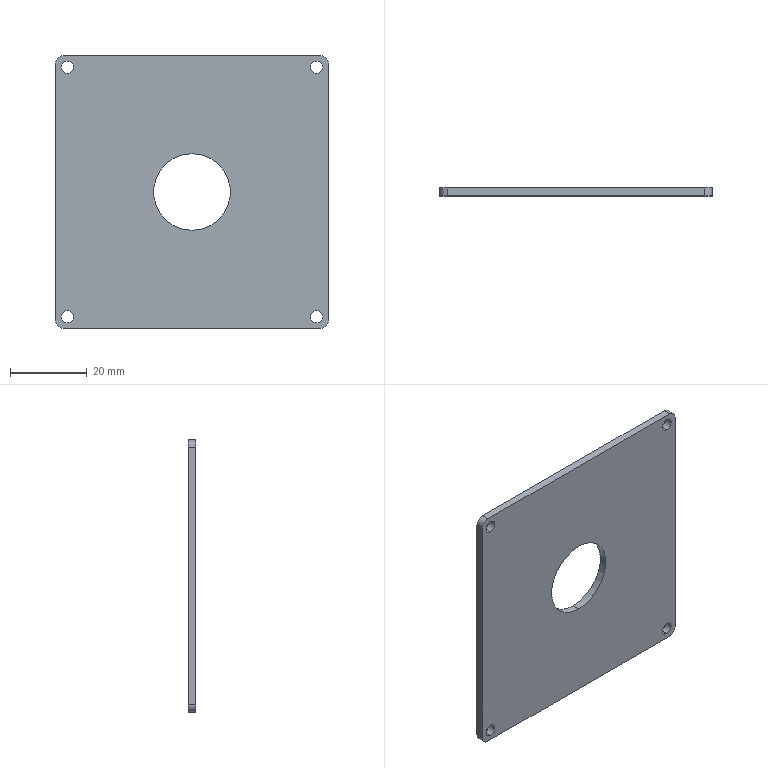Part | SolidWorks | features Extrusion 1, ICE 1 | 1 solid | 20 faces | box 71 x 2 x 71 mm | volume 9382 mm3 | cylinder 14 | plane 6 | commonest cylinder face diameters 3.2 x8 4 x4 20 x2
STEP:
#1=CARTESIAN_POINT('',(0.,0.,10.));
#2=VERTEX_POINT('',#1);
#3=CARTESIAN_POINT('',(0.,0.,-10.));
#4=VERTEX_POINT('',#3);
#5=CARTESIAN_POINT('',(0.,0.,0.));
#6=DIRECTION('',(0.,-1.,0.));
#7=DIRECTION('',(0.,0.,-1.));
#8=AXIS2_PLACEMENT_3D('',#5,#6,#7);
#9=CIRCLE('',#8,10.);
#10=EDGE_CURVE('',#2,#4,#9,.T.);
#11=ORIENTED_EDGE('',*,*,#10,.T.);
#12=CARTESIAN_POINT('',(0.,2.,-10.));
#13=VERTEX_POINT('',#12);
#14=CARTESIAN_POINT('',(0.,-8.,-10.));
#15=DIRECTION('',(0.,1.,0.));
#16=VECTOR('',#15,1000.);
#17=LINE('',#14,#16);
#18=EDGE_CURVE('',#4,#13,#17,.T.);
#19=ORIENTED_EDGE('',*,*,#18,.T.);
#20=CARTESIAN_POINT('',(0.,2.,10.));
#21=VERTEX_POINT('',#20);
#22=CARTESIAN_POINT('',(0.,2.,0.));
#23=DIRECTION('',(0.,1.,0.));
#24=DIRECTION('',(0.,0.,1.));
#25=AXIS2_PLACEMENT_3D('',#22,#23,#24);
#26=CIRCLE('',#25,10.);
#27=EDGE_CURVE('',#13,#21,#26,.T.);
#28=ORIENTED_EDGE('',*,*,#27,.T.);
#29=CARTESIAN_POINT('',(0.,-8.,10.));
#30=DIRECTION('',(0.,1.,0.));
#31=VECTOR('',#30,1000.);
#32=LINE('',#29,#31);
#33=EDGE_CURVE('',#2,#21,#32,.T.);
#34=ORIENTED_EDGE('',*,*,#33,.F.);
#35=EDGE_LOOP('',(#11,#19,#28,#34));
#36=FACE_OUTER_BOUND('',#35,.T.);
#37=CARTESIAN_POINT('',(0.,-8.,0.));
#38=DIRECTION('',(0.,1.,0.));
#39=DIRECTION('',(0.,0.,1.));
#40=AXIS2_PLACEMENT_3D('',#37,#38,#39);
#41=CYLINDRICAL_SURFACE('',#40,10.);
#42=ADVANCED_FACE('',(#36),#41,.F.);
#43=CARTESIAN_POINT('',(-32.5,2.,30.9));
#44=VERTEX_POINT('',#43);
#45=CARTESIAN_POINT('',(-32.5,2.,34.1));
#46=VERTEX_POINT('',#45);
#47=CARTESIAN_POINT('',(-32.5,2.,32.5));
#48=DIRECTION('',(0.,1.,0.));
#49=DIRECTION('',(0.,0.,1.));
#50=AXIS2_PLACEMENT_3D('',#47,#48,#49);
#51=CIRCLE('',#50,1.6);
#52=EDGE_CURVE('',#44,#46,#51,.T.);
#53=ORIENTED_EDGE('',*,*,#52,.T.);
#54=CARTESIAN_POINT('',(-32.5,0.,34.1));
#55=VERTEX_POINT('',#54);
#56=CARTESIAN_POINT('',(-32.5,2.,34.1));
#57=DIRECTION('',(0.,-1.,0.));
#58=VECTOR('',#57,1000.);
#59=LINE('',#56,#58);
#60=EDGE_CURVE('',#46,#55,#59,.T.);
#61=ORIENTED_EDGE('',*,*,#60,.T.);
#62=CARTESIAN_POINT('',(-32.5,0.,30.9));
#63=VERTEX_POINT('',#62);
#64=CARTESIAN_POINT('',(-32.5,0.,32.5));
#65=DIRECTION('',(0.,1.,0.));
#66=DIRECTION('',(0.,0.,1.));
#67=AXIS2_PLACEMENT_3D('',#64,#65,#66);
#68=CIRCLE('',#67,1.6);
#69=EDGE_CURVE('',#63,#55,#68,.T.);
#70=ORIENTED_EDGE('',*,*,#69,.F.);
#71=CARTESIAN_POINT('',(-32.5,2.,30.9));
#72=DIRECTION('',(0.,-1.,0.));
#73=VECTOR('',#72,1000.);
#74=LINE('',#71,#73);
#75=EDGE_CURVE('',#44,#63,#74,.T.);
#76=ORIENTED_EDGE('',*,*,#75,.F.);
#77=EDGE_LOOP('',(#53,#61,#70,#76));
#78=FACE_OUTER_BOUND('',#77,.T.);
#79=CARTESIAN_POINT('',(-32.5,2.,32.5));
#80=DIRECTION('',(0.,-1.,0.));
#81=DIRECTION('',(0.,0.,-1.));
#82=AXIS2_PLACEMENT_3D('',#79,#80,#81);
#83=CYLINDRICAL_SURFACE('',#82,1.6);
#84=ADVANCED_FACE('',(#78),#83,.F.);
#85=CARTESIAN_POINT('',(32.5,2.,30.9));
#86=VERTEX_POINT('',#85);
#87=CARTESIAN_POINT('',(32.5,2.,34.1));
#88=VERTEX_POINT('',#87);
#89=CARTESIAN_POINT('',(32.5,2.,32.5));
#90=DIRECTION('',(0.,1.,0.));
#91=DIRECTION('',(0.,0.,1.));
#92=AXIS2_PLACEMENT_3D('',#89,#90,#91);
#93=CIRCLE('',#92,1.6);
#94=EDGE_CURVE('',#86,#88,#93,.T.);
#95=ORIENTED_EDGE('',*,*,#94,.T.);
#96=CARTESIAN_POINT('',(32.5,0.,34.1));
#97=VERTEX_POINT('',#96);
#98=CARTESIAN_POINT('',(32.5,2.,34.1));
#99=DIRECTION('',(0.,-1.,0.));
#100=VECTOR('',#99,1000.);
#101=LINE('',#98,#100);
#102=EDGE_CURVE('',#88,#97,#101,.T.);
#103=ORIENTED_EDGE('',*,*,#102,.T.);
#104=CARTESIAN_POINT('',(32.5,0.,30.9));
#105=VERTEX_POINT('',#104);
#106=CARTESIAN_POINT('',(32.5,0.,32.5));
#107=DIRECTION('',(0.,1.,0.));
#108=DIRECTION('',(0.,0.,1.));
#109=AXIS2_PLACEMENT_3D('',#106,#107,#108);
#110=CIRCLE('',#109,1.6);
#111=EDGE_CURVE('',#105,#97,#110,.T.);
#112=ORIENTED_EDGE('',*,*,#111,.F.);
#113=CARTESIAN_POINT('',(32.5,2.,30.9));
#114=DIRECTION('',(0.,-1.,0.));
#115=VECTOR('',#114,1000.);
#116=LINE('',#113,#115);
#117=EDGE_CURVE('',#86,#105,#116,.T.);
#118=ORIENTED_EDGE('',*,*,#117,.F.);
#119=EDGE_LOOP('',(#95,#103,#112,#118));
#120=FACE_OUTER_BOUND('',#119,.T.);
#121=CARTESIAN_POINT('',(32.5,2.,32.5));
#122=DIRECTION('',(0.,-1.,0.));
#123=DIRECTION('',(0.,0.,-1.));
#124=AXIS2_PLACEMENT_3D('',#121,#122,#123);
#125=CYLINDRICAL_SURFACE('',#124,1.6);
#126=ADVANCED_FACE('',(#120),#125,.F.);
#127=CARTESIAN_POINT('',(32.5,2.,-34.1));
#128=VERTEX_POINT('',#127);
#129=CARTESIAN_POINT('',(32.5,2.,-30.9));
#130=VERTEX_POINT('',#129);
#131=CARTESIAN_POINT('',(32.5,2.,-32.5));
#132=DIRECTION('',(0.,1.,0.));
#133=DIRECTION('',(0.,0.,1.));
#134=AXIS2_PLACEMENT_3D('',#131,#132,#133);
#135=CIRCLE('',#134,1.6);
#136=EDGE_CURVE('',#128,#130,#135,.T.);
#137=ORIENTED_EDGE('',*,*,#136,.T.);
#138=CARTESIAN_POINT('',(32.5,0.,-30.9));
#139=VERTEX_POINT('',#138);
#140=CARTESIAN_POINT('',(32.5,2.,-30.9));
#141=DIRECTION('',(0.,-1.,0.));
#142=VECTOR('',#141,1000.);
#143=LINE('',#140,#142);
#144=EDGE_CURVE('',#130,#139,#143,.T.);
#145=ORIENTED_EDGE('',*,*,#144,.T.);
#146=CARTESIAN_POINT('',(32.5,0.,-34.1));
#147=VERTEX_POINT('',#146);
#148=CARTESIAN_POINT('',(32.5,0.,-32.5));
#149=DIRECTION('',(0.,1.,0.));
#150=DIRECTION('',(0.,0.,1.));
#151=AXIS2_PLACEMENT_3D('',#148,#149,#150);
#152=CIRCLE('',#151,1.6);
#153=EDGE_CURVE('',#147,#139,#152,.T.);
#154=ORIENTED_EDGE('',*,*,#153,.F.);
#155=CARTESIAN_POINT('',(32.5,2.,-34.1));
#156=DIRECTION('',(0.,-1.,0.));
#157=VECTOR('',#156,1000.);
#158=LINE('',#155,#157);
#159=EDGE_CURVE('',#128,#147,#158,.T.);
#160=ORIENTED_EDGE('',*,*,#159,.F.);
#161=EDGE_LOOP('',(#137,#145,#154,#160));
#162=FACE_OUTER_BOUND('',#161,.T.);
#163=CARTESIAN_POINT('',(32.5,2.,-32.5));
#164=DIRECTION('',(0.,-1.,0.));
#165=DIRECTION('',(0.,0.,-1.));
#166=AXIS2_PLACEMENT_3D('',#163,#164,#165);
#167=CYLINDRICAL_SURFACE('',#166,1.6);
#168=ADVANCED_FACE('',(#162),#167,.F.);
#169=CARTESIAN_POINT('',(-32.5,2.,-34.1));
#170=VERTEX_POINT('',#169);
#171=CARTESIAN_POINT('',(-32.5,2.,-30.9));
#172=VERTEX_POINT('',#171);
#173=CARTESIAN_POINT('',(-32.5,2.,-32.5));
#174=DIRECTION('',(0.,1.,0.));
#175=DIRECTION('',(0.,0.,1.));
#176=AXIS2_PLACEMENT_3D('',#173,#174,#175);
#177=CIRCLE('',#176,1.6);
#178=EDGE_CURVE('',#170,#172,#177,.T.);
#179=ORIENTED_EDGE('',*,*,#178,.T.);
#180=CARTESIAN_POINT('',(-32.5,0.,-30.9));
#181=VERTEX_POINT('',#180);
#182=CARTESIAN_POINT('',(-32.5,2.,-30.9));
#183=DIRECTION('',(0.,-1.,0.));
#184=VECTOR('',#183,1000.);
#185=LINE('',#182,#184);
#186=EDGE_CURVE('',#172,#181,#185,.T.);
#187=ORIENTED_EDGE('',*,*,#186,.T.);
#188=CARTESIAN_POINT('',(-32.5,0.,-34.1));
#189=VERTEX_POINT('',#188);
#190=CARTESIAN_POINT('',(-32.5,0.,-32.5));
#191=DIRECTION('',(0.,1.,0.));
#192=DIRECTION('',(0.,0.,1.));
#193=AXIS2_PLACEMENT_3D('',#190,#191,#192);
#194=CIRCLE('',#193,1.6);
#195=EDGE_CURVE('',#189,#181,#194,.T.);
#196=ORIENTED_EDGE('',*,*,#195,.F.);
#197=CARTESIAN_POINT('',(-32.5,2.,-34.1));
#198=DIRECTION('',(0.,-1.,0.));
#199=VECTOR('',#198,1000.);
#200=LINE('',#197,#199);
#201=EDGE_CURVE('',#170,#189,#200,.T.);
#202=ORIENTED_EDGE('',*,*,#201,.F.);
#203=EDGE_LOOP('',(#179,#187,#196,#202));
#204=FACE_OUTER_BOUND('',#203,.T.);
#205=CARTESIAN_POINT('',(-32.5,2.,-32.5));
#206=DIRECTION('',(0.,-1.,0.));
#207=DIRECTION('',(0.,0.,-1.));
#208=AXIS2_PLACEMENT_3D('',#205,#206,#207);
#209=CYLINDRICAL_SURFACE('',#208,1.6);
#210=ADVANCED_FACE('',(#204),#209,.F.);
#211=CARTESIAN_POINT('',(0.,2.,0.));
#212=DIRECTION('',(0.,1.,0.));
#213=DIRECTION('',(0.,0.,1.));
#214=AXIS2_PLACEMENT_3D('',#211,#212,#213);
#215=CIRCLE('',#214,10.);
#216=EDGE_CURVE('',#21,#13,#215,.T.);
#217=ORIENTED_EDGE('',*,*,#216,.F.);
#218=ORIENTED_EDGE('',*,*,#27,.F.);
#219=EDGE_LOOP('',(#217,#218));
#220=FACE_BOUND('',#219,.T.);
#221=CARTESIAN_POINT('',(-35.5,2.,33.5));
#222=VERTEX_POINT('',#221);
#223=CARTESIAN_POINT('',(-33.5,2.,35.5));
#224=VERTEX_POINT('',#223);
#225=CARTESIAN_POINT('',(-33.5,2.,33.5));
#226=DIRECTION('',(0.,1.,0.));
#227=DIRECTION('',(0.,0.,-1.));
#228=AXIS2_PLACEMENT_3D('',#225,#226,#227);
#229=CIRCLE('',#228,2.);
#230=EDGE_CURVE('',#222,#224,#229,.T.);
#231=ORIENTED_EDGE('',*,*,#230,.T.);
#232=CARTESIAN_POINT('',(33.5,2.,35.5));
#233=VERTEX_POINT('',#232);
#234=CARTESIAN_POINT('',(-33.5,2.,35.5));
#235=DIRECTION('',(1.,0.,0.));
#236=VECTOR('',#235,1000.);
#237=LINE('',#234,#236);
#238=EDGE_CURVE('',#224,#233,#237,.T.);
#239=ORIENTED_EDGE('',*,*,#238,.T.);
#240=CARTESIAN_POINT('',(35.5,2.,33.5));
#241=VERTEX_POINT('',#240);
#242=CARTESIAN_POINT('',(33.5,2.,33.5));
#243=DIRECTION('',(0.,1.,0.));
#244=DIRECTION('',(0.,0.,1.));
#245=AXIS2_PLACEMENT_3D('',#242,#243,#244);
#246=CIRCLE('',#245,2.);
#247=EDGE_CURVE('',#233,#241,#246,.T.);
#248=ORIENTED_EDGE('',*,*,#247,.T.);
#249=CARTESIAN_POINT('',(35.5,2.,-33.5));
#250=VERTEX_POINT('',#249);
#251=CARTESIAN_POINT('',(35.5,2.,33.5));
#252=DIRECTION('',(0.,0.,-1.));
#253=VECTOR('',#252,1000.);
#254=LINE('',#251,#253);
#255=EDGE_CURVE('',#241,#250,#254,.T.);
#256=ORIENTED_EDGE('',*,*,#255,.T.);
#257=CARTESIAN_POINT('',(33.5,2.,-35.5));
#258=VERTEX_POINT('',#257);
#259=CARTESIAN_POINT('',(33.5,2.,-33.5));
#260=DIRECTION('',(0.,1.,0.));
#261=DIRECTION('',(0.,0.,-1.));
#262=AXIS2_PLACEMENT_3D('',#259,#260,#261);
#263=CIRCLE('',#262,2.);
#264=EDGE_CURVE('',#250,#258,#263,.T.);
#265=ORIENTED_EDGE('',*,*,#264,.T.);
#266=CARTESIAN_POINT('',(-33.5,2.,-35.5));
#267=VERTEX_POINT('',#266);
#268=CARTESIAN_POINT('',(-33.5,2.,-35.5));
#269=DIRECTION('',(-1.,0.,0.));
#270=VECTOR('',#269,1000.);
#271=LINE('',#268,#270);
#272=EDGE_CURVE('',#258,#267,#271,.T.);
#273=ORIENTED_EDGE('',*,*,#272,.T.);
#274=CARTESIAN_POINT('',(-35.5,2.,-33.5));
#275=VERTEX_POINT('',#274);
#276=CARTESIAN_POINT('',(-33.5,2.,-33.5));
#277=DIRECTION('',(0.,1.,0.));
#278=DIRECTION('',(0.,0.,-1.));
#279=AXIS2_PLACEMENT_3D('',#276,#277,#278);
#280=CIRCLE('',#279,2.);
#281=EDGE_CURVE('',#267,#275,#280,.T.);
#282=ORIENTED_EDGE('',*,*,#281,.T.);
#283=CARTESIAN_POINT('',(-35.5,2.,33.5));
#284=DIRECTION('',(0.,0.,1.));
#285=VECTOR('',#284,1000.);
#286=LINE('',#283,#285);
#287=EDGE_CURVE('',#275,#222,#286,.T.);
#288=ORIENTED_EDGE('',*,*,#287,.T.);
#289=EDGE_LOOP('',(#231,#239,#248,#256,#265,#273,#282,#288));
#290=FACE_OUTER_BOUND('',#289,.T.);
#291=ORIENTED_EDGE('',*,*,#178,.F.);
#292=CARTESIAN_POINT('',(-32.5,2.,-32.5));
#293=DIRECTION('',(0.,1.,0.));
#294=DIRECTION('',(0.,0.,1.));
#295=AXIS2_PLACEMENT_3D('',#292,#293,#294);
#296=CIRCLE('',#295,1.6);
#297=EDGE_CURVE('',#172,#170,#296,.T.);
#298=ORIENTED_EDGE('',*,*,#297,.F.);
#299=EDGE_LOOP('',(#291,#298));
#300=FACE_BOUND('',#299,.T.);
#301=ORIENTED_EDGE('',*,*,#136,.F.);
#302=CARTESIAN_POINT('',(32.5,2.,-32.5));
#303=DIRECTION('',(0.,1.,0.));
#304=DIRECTION('',(0.,0.,1.));
#305=AXIS2_PLACEMENT_3D('',#302,#303,#304);
#306=CIRCLE('',#305,1.6);
#307=EDGE_CURVE('',#130,#128,#306,.T.);
#308=ORIENTED_EDGE('',*,*,#307,.F.);
#309=EDGE_LOOP('',(#301,#308));
#310=FACE_BOUND('',#309,.T.);
#311=ORIENTED_EDGE('',*,*,#94,.F.);
#312=CARTESIAN_POINT('',(32.5,2.,32.5));
#313=DIRECTION('',(0.,1.,0.));
#314=DIRECTION('',(0.,0.,1.));
#315=AXIS2_PLACEMENT_3D('',#312,#313,#314);
#316=CIRCLE('',#315,1.6);
#317=EDGE_CURVE('',#88,#86,#316,.T.);
#318=ORIENTED_EDGE('',*,*,#317,.F.);
#319=EDGE_LOOP('',(#311,#318));
#320=FACE_BOUND('',#319,.T.);
#321=ORIENTED_EDGE('',*,*,#52,.F.);
#322=CARTESIAN_POINT('',(-32.5,2.,32.5));
#323=DIRECTION('',(0.,1.,0.));
#324=DIRECTION('',(0.,0.,1.));
#325=AXIS2_PLACEMENT_3D('',#322,#323,#324);
#326=CIRCLE('',#325,1.6);
#327=EDGE_CURVE('',#46,#44,#326,.T.);
#328=ORIENTED_EDGE('',*,*,#327,.F.);
#329=EDGE_LOOP('',(#321,#328));
#330=FACE_BOUND('',#329,.T.);
#331=CARTESIAN_POINT('',(-33.5,2.,33.5));
#332=DIRECTION('',(0.,-1.,0.));
#333=DIRECTION('',(0.,0.,-1.));
#334=AXIS2_PLACEMENT_3D('',#331,#332,#333);
#335=PLANE('',#334);
#336=ADVANCED_FACE('',(#220,#290,#300,#310,#320,#330),#335,.F.);
#337=ORIENTED_EDGE('',*,*,#10,.F.);
#338=CARTESIAN_POINT('',(0.,0.,0.));
#339=DIRECTION('',(0.,-1.,0.));
#340=DIRECTION('',(0.,0.,-1.));
#341=AXIS2_PLACEMENT_3D('',#338,#339,#340);
#342=CIRCLE('',#341,10.);
#343=EDGE_CURVE('',#4,#2,#342,.T.);
#344=ORIENTED_EDGE('',*,*,#343,.F.);
#345=EDGE_LOOP('',(#337,#344));
#346=FACE_BOUND('',#345,.T.);
#347=ORIENTED_EDGE('',*,*,#111,.T.);
#348=CARTESIAN_POINT('',(32.5,0.,32.5));
#349=DIRECTION('',(0.,1.,0.));
#350=DIRECTION('',(0.,0.,1.));
#351=AXIS2_PLACEMENT_3D('',#348,#349,#350);
#352=CIRCLE('',#351,1.6);
#353=EDGE_CURVE('',#97,#105,#352,.T.);
#354=ORIENTED_EDGE('',*,*,#353,.T.);
#355=EDGE_LOOP('',(#347,#354));
#356=FACE_BOUND('',#355,.T.);
#357=ORIENTED_EDGE('',*,*,#195,.T.);
#358=CARTESIAN_POINT('',(-32.5,0.,-32.5));
#359=DIRECTION('',(0.,1.,0.));
#360=DIRECTION('',(0.,0.,1.));
#361=AXIS2_PLACEMENT_3D('',#358,#359,#360);
#362=CIRCLE('',#361,1.6);
#363=EDGE_CURVE('',#181,#189,#362,.T.);
#364=ORIENTED_EDGE('',*,*,#363,.T.);
#365=EDGE_LOOP('',(#357,#364));
#366=FACE_BOUND('',#365,.T.);
#367=CARTESIAN_POINT('',(-35.5,0.,33.5));
#368=VERTEX_POINT('',#367);
#369=CARTESIAN_POINT('',(-33.5,0.,35.5));
#370=VERTEX_POINT('',#369);
#371=CARTESIAN_POINT('',(-33.5,0.,33.5));
#372=DIRECTION('',(0.,1.,0.));
#373=DIRECTION('',(0.,0.,-1.));
#374=AXIS2_PLACEMENT_3D('',#371,#372,#373);
#375=CIRCLE('',#374,2.);
#376=EDGE_CURVE('',#368,#370,#375,.T.);
#377=ORIENTED_EDGE('',*,*,#376,.F.);
#378=CARTESIAN_POINT('',(-35.5,0.,-33.5));
#379=VERTEX_POINT('',#378);
#380=CARTESIAN_POINT('',(-35.5,0.,33.5));
#381=DIRECTION('',(0.,0.,1.));
#382=VECTOR('',#381,1000.);
#383=LINE('',#380,#382);
#384=EDGE_CURVE('',#379,#368,#383,.T.);
#385=ORIENTED_EDGE('',*,*,#384,.F.);
#386=CARTESIAN_POINT('',(-33.5,0.,-35.5));
#387=VERTEX_POINT('',#386);
#388=CARTESIAN_POINT('',(-33.5,0.,-33.5));
#389=DIRECTION('',(0.,1.,0.));
#390=DIRECTION('',(0.,0.,-1.));
#391=AXIS2_PLACEMENT_3D('',#388,#389,#390);
#392=CIRCLE('',#391,2.);
#393=EDGE_CURVE('',#387,#379,#392,.T.);
#394=ORIENTED_EDGE('',*,*,#393,.F.);
#395=CARTESIAN_POINT('',(33.5,0.,-35.5));
#396=VERTEX_POINT('',#395);
#397=CARTESIAN_POINT('',(-33.5,0.,-35.5));
#398=DIRECTION('',(-1.,0.,0.));
#399=VECTOR('',#398,1000.);
#400=LINE('',#397,#399);
#401=EDGE_CURVE('',#396,#387,#400,.T.);
#402=ORIENTED_EDGE('',*,*,#401,.F.);
#403=CARTESIAN_POINT('',(35.5,0.,-33.5));
#404=VERTEX_POINT('',#403);
#405=CARTESIAN_POINT('',(33.5,0.,-33.5));
#406=DIRECTION('',(0.,1.,0.));
#407=DIRECTION('',(0.,0.,-1.));
#408=AXIS2_PLACEMENT_3D('',#405,#406,#407);
#409=CIRCLE('',#408,2.);
#410=EDGE_CURVE('',#404,#396,#409,.T.);
#411=ORIENTED_EDGE('',*,*,#410,.F.);
#412=CARTESIAN_POINT('',(35.5,0.,33.5));
#413=VERTEX_POINT('',#412);
#414=CARTESIAN_POINT('',(35.5,0.,33.5));
#415=DIRECTION('',(0.,0.,-1.));
#416=VECTOR('',#415,1000.);
#417=LINE('',#414,#416);
#418=EDGE_CURVE('',#413,#404,#417,.T.);
#419=ORIENTED_EDGE('',*,*,#418,.F.);
#420=CARTESIAN_POINT('',(33.5,0.,35.5));
#421=VERTEX_POINT('',#420);
#422=CARTESIAN_POINT('',(33.5,0.,33.5));
#423=DIRECTION('',(0.,1.,0.));
#424=DIRECTION('',(0.,0.,1.));
#425=AXIS2_PLACEMENT_3D('',#422,#423,#424);
#426=CIRCLE('',#425,2.);
#427=EDGE_CURVE('',#421,#413,#426,.T.);
#428=ORIENTED_EDGE('',*,*,#427,.F.);
#429=CARTESIAN_POINT('',(-33.5,0.,35.5));
#430=DIRECTION('',(1.,0.,0.));
#431=VECTOR('',#430,1000.);
#432=LINE('',#429,#431);
#433=EDGE_CURVE('',#370,#421,#432,.T.);
#434=ORIENTED_EDGE('',*,*,#433,.F.);
#435=EDGE_LOOP('',(#377,#385,#394,#402,#411,#419,#428,#434));
#436=FACE_OUTER_BOUND('',#435,.T.);
#437=ORIENTED_EDGE('',*,*,#153,.T.);
#438=CARTESIAN_POINT('',(32.5,0.,-32.5));
#439=DIRECTION('',(0.,1.,0.));
#440=DIRECTION('',(0.,0.,1.));
#441=AXIS2_PLACEMENT_3D('',#438,#439,#440);
#442=CIRCLE('',#441,1.6);
#443=EDGE_CURVE('',#139,#147,#442,.T.);
#444=ORIENTED_EDGE('',*,*,#443,.T.);
#445=EDGE_LOOP('',(#437,#444));
#446=FACE_BOUND('',#445,.T.);
#447=ORIENTED_EDGE('',*,*,#69,.T.);
#448=CARTESIAN_POINT('',(-32.5,0.,32.5));
#449=DIRECTION('',(0.,1.,0.));
#450=DIRECTION('',(0.,0.,1.));
#451=AXIS2_PLACEMENT_3D('',#448,#449,#450);
#452=CIRCLE('',#451,1.6);
#453=EDGE_CURVE('',#55,#63,#452,.T.);
#454=ORIENTED_EDGE('',*,*,#453,.T.);
#455=EDGE_LOOP('',(#447,#454));
#456=FACE_BOUND('',#455,.T.);
#457=CARTESIAN_POINT('',(-33.5,0.,33.5));
#458=DIRECTION('',(0.,-1.,0.));
#459=DIRECTION('',(0.,0.,-1.));
#460=AXIS2_PLACEMENT_3D('',#457,#458,#459);
#461=PLANE('',#460);
#462=ADVANCED_FACE('',(#346,#356,#366,#436,#446,#456),#461,.T.);
#463=ORIENTED_EDGE('',*,*,#376,.T.);
#464=CARTESIAN_POINT('',(-33.5,2.,35.5));
#465=DIRECTION('',(0.,-1.,0.));
#466=VECTOR('',#465,1000.);
#467=LINE('',#464,#466);
#468=EDGE_CURVE('',#224,#370,#467,.T.);
#469=ORIENTED_EDGE('',*,*,#468,.F.);
#470=ORIENTED_EDGE('',*,*,#230,.F.);
#471=CARTESIAN_POINT('',(-35.5,2.,33.5));
#472=DIRECTION('',(0.,-1.,0.));
#473=VECTOR('',#472,1000.);
#474=LINE('',#471,#473);
#475=EDGE_CURVE('',#222,#368,#474,.T.);
#476=ORIENTED_EDGE('',*,*,#475,.T.);
#477=EDGE_LOOP('',(#463,#469,#470,#476));
#478=FACE_OUTER_BOUND('',#477,.T.);
#479=CARTESIAN_POINT('',(-33.5,2.,33.5));
#480=DIRECTION('',(0.,-1.,0.));
#481=DIRECTION('',(0.,0.,-1.));
#482=AXIS2_PLACEMENT_3D('',#479,#480,#481);
#483=CYLINDRICAL_SURFACE('',#482,2.);
#484=ADVANCED_FACE('',(#478),#483,.T.);
#485=ORIENTED_EDGE('',*,*,#433,.T.);
#486=CARTESIAN_POINT('',(33.5,2.,35.5));
#487=DIRECTION('',(0.,-1.,0.));
#488=VECTOR('',#487,1000.);
#489=LINE('',#486,#488);
#490=EDGE_CURVE('',#233,#421,#489,.T.);
#491=ORIENTED_EDGE('',*,*,#490,.F.);
#492=ORIENTED_EDGE('',*,*,#238,.F.);
#493=ORIENTED_EDGE('',*,*,#468,.T.);
#494=EDGE_LOOP('',(#485,#491,#492,#493));
#495=FACE_OUTER_BOUND('',#494,.T.);
#496=CARTESIAN_POINT('',(-33.5,2.,35.5));
#497=DIRECTION('',(0.,0.,-1.));
#498=DIRECTION('',(-1.,0.,0.));
#499=AXIS2_PLACEMENT_3D('',#496,#497,#498);
#500=PLANE('',#499);
#501=ADVANCED_FACE('',(#495),#500,.F.);
#502=ORIENTED_EDGE('',*,*,#427,.T.);
#503=CARTESIAN_POINT('',(35.5,2.,33.5));
#504=DIRECTION('',(0.,-1.,0.));
#505=VECTOR('',#504,1000.);
#506=LINE('',#503,#505);
#507=EDGE_CURVE('',#241,#413,#506,.T.);
#508=ORIENTED_EDGE('',*,*,#507,.F.);
#509=ORIENTED_EDGE('',*,*,#247,.F.);
#510=ORIENTED_EDGE('',*,*,#490,.T.);
#511=EDGE_LOOP('',(#502,#508,#509,#510));
#512=FACE_OUTER_BOUND('',#511,.T.);
#513=CARTESIAN_POINT('',(33.5,2.,33.5));
#514=DIRECTION('',(0.,-1.,0.));
#515=DIRECTION('',(0.,0.,-1.));
#516=AXIS2_PLACEMENT_3D('',#513,#514,#515);
#517=CYLINDRICAL_SURFACE('',#516,2.);
#518=ADVANCED_FACE('',(#512),#517,.T.);
#519=ORIENTED_EDGE('',*,*,#418,.T.);
#520=CARTESIAN_POINT('',(35.5,2.,-33.5));
#521=DIRECTION('',(0.,-1.,0.));
#522=VECTOR('',#521,1000.);
#523=LINE('',#520,#522);
#524=EDGE_CURVE('',#250,#404,#523,.T.);
#525=ORIENTED_EDGE('',*,*,#524,.F.);
#526=ORIENTED_EDGE('',*,*,#255,.F.);
#527=ORIENTED_EDGE('',*,*,#507,.T.);
#528=EDGE_LOOP('',(#519,#525,#526,#527));
#529=FACE_OUTER_BOUND('',#528,.T.);
#530=CARTESIAN_POINT('',(35.5,2.,33.5));
#531=DIRECTION('',(-1.,0.,0.));
#532=DIRECTION('',(0.,0.,1.));
#533=AXIS2_PLACEMENT_3D('',#530,#531,#532);
#534=PLANE('',#533);
#535=ADVANCED_FACE('',(#529),#534,.F.);
#536=ORIENTED_EDGE('',*,*,#410,.T.);
#537=CARTESIAN_POINT('',(33.5,2.,-35.5));
#538=DIRECTION('',(0.,-1.,0.));
#539=VECTOR('',#538,1000.);
#540=LINE('',#537,#539);
#541=EDGE_CURVE('',#258,#396,#540,.T.);
#542=ORIENTED_EDGE('',*,*,#541,.F.);
#543=ORIENTED_EDGE('',*,*,#264,.F.);
#544=ORIENTED_EDGE('',*,*,#524,.T.);
#545=EDGE_LOOP('',(#536,#542,#543,#544));
#546=FACE_OUTER_BOUND('',#545,.T.);
#547=CARTESIAN_POINT('',(33.5,2.,-33.5));
#548=DIRECTION('',(0.,-1.,0.));
#549=DIRECTION('',(0.,0.,-1.));
#550=AXIS2_PLACEMENT_3D('',#547,#548,#549);
#551=CYLINDRICAL_SURFACE('',#550,2.);
#552=ADVANCED_FACE('',(#546),#551,.T.);
#553=ORIENTED_EDGE('',*,*,#401,.T.);
#554=CARTESIAN_POINT('',(-33.5,2.,-35.5));
#555=DIRECTION('',(0.,-1.,0.));
#556=VECTOR('',#555,1000.);
#557=LINE('',#554,#556);
#558=EDGE_CURVE('',#267,#387,#557,.T.);
#559=ORIENTED_EDGE('',*,*,#558,.F.);
#560=ORIENTED_EDGE('',*,*,#272,.F.);
#561=ORIENTED_EDGE('',*,*,#541,.T.);
#562=EDGE_LOOP('',(#553,#559,#560,#561));
#563=FACE_OUTER_BOUND('',#562,.T.);
#564=CARTESIAN_POINT('',(-33.5,2.,-35.5));
#565=DIRECTION('',(0.,0.,1.));
#566=DIRECTION('',(1.,0.,0.));
#567=AXIS2_PLACEMENT_3D('',#564,#565,#566);
#568=PLANE('',#567);
#569=ADVANCED_FACE('',(#563),#568,.F.);
#570=ORIENTED_EDGE('',*,*,#393,.T.);
#571=CARTESIAN_POINT('',(-35.5,2.,-33.5));
#572=DIRECTION('',(0.,-1.,0.));
#573=VECTOR('',#572,1000.);
#574=LINE('',#571,#573);
#575=EDGE_CURVE('',#275,#379,#574,.T.);
#576=ORIENTED_EDGE('',*,*,#575,.F.);
#577=ORIENTED_EDGE('',*,*,#281,.F.);
#578=ORIENTED_EDGE('',*,*,#558,.T.);
#579=EDGE_LOOP('',(#570,#576,#577,#578));
#580=FACE_OUTER_BOUND('',#579,.T.);
#581=CARTESIAN_POINT('',(-33.5,2.,-33.5));
#582=DIRECTION('',(0.,-1.,0.));
#583=DIRECTION('',(0.,0.,-1.));
#584=AXIS2_PLACEMENT_3D('',#581,#582,#583);
#585=CYLINDRICAL_SURFACE('',#584,2.);
#586=ADVANCED_FACE('',(#580),#585,.T.);
#587=ORIENTED_EDGE('',*,*,#384,.T.);
#588=ORIENTED_EDGE('',*,*,#475,.F.);
#589=ORIENTED_EDGE('',*,*,#287,.F.);
#590=ORIENTED_EDGE('',*,*,#575,.T.);
#591=EDGE_LOOP('',(#587,#588,#589,#590));
#592=FACE_OUTER_BOUND('',#591,.T.);
#593=CARTESIAN_POINT('',(-35.5,2.,33.5));
#594=DIRECTION('',(1.,0.,0.));
#595=DIRECTION('',(0.,0.,-1.));
#596=AXIS2_PLACEMENT_3D('',#593,#594,#595);
#597=PLANE('',#596);
#598=ADVANCED_FACE('',(#592),#597,.F.);
#599=ORIENTED_EDGE('',*,*,#186,.F.);
#600=ORIENTED_EDGE('',*,*,#297,.T.);
#601=ORIENTED_EDGE('',*,*,#201,.T.);
#602=ORIENTED_EDGE('',*,*,#363,.F.);
#603=EDGE_LOOP('',(#599,#600,#601,#602));
#604=FACE_OUTER_BOUND('',#603,.T.);
#605=CARTESIAN_POINT('',(-32.5,2.,-32.5));
#606=DIRECTION('',(0.,-1.,0.));
#607=DIRECTION('',(0.,0.,-1.));
#608=AXIS2_PLACEMENT_3D('',#605,#606,#607);
#609=CYLINDRICAL_SURFACE('',#608,1.6);
#610=ADVANCED_FACE('',(#604),#609,.F.);
#611=ORIENTED_EDGE('',*,*,#144,.F.);
#612=ORIENTED_EDGE('',*,*,#307,.T.);
#613=ORIENTED_EDGE('',*,*,#159,.T.);
#614=ORIENTED_EDGE('',*,*,#443,.F.);
#615=EDGE_LOOP('',(#611,#612,#613,#614));
#616=FACE_OUTER_BOUND('',#615,.T.);
#617=CARTESIAN_POINT('',(32.5,2.,-32.5));
#618=DIRECTION('',(0.,-1.,0.));
#619=DIRECTION('',(0.,0.,-1.));
#620=AXIS2_PLACEMENT_3D('',#617,#618,#619);
#621=CYLINDRICAL_SURFACE('',#620,1.6);
#622=ADVANCED_FACE('',(#616),#621,.F.);
#623=ORIENTED_EDGE('',*,*,#102,.F.);
#624=ORIENTED_EDGE('',*,*,#317,.T.);
#625=ORIENTED_EDGE('',*,*,#117,.T.);
#626=ORIENTED_EDGE('',*,*,#353,.F.);
#627=EDGE_LOOP('',(#623,#624,#625,#626));
#628=FACE_OUTER_BOUND('',#627,.T.);
#629=CARTESIAN_POINT('',(32.5,2.,32.5));
#630=DIRECTION('',(0.,-1.,0.));
#631=DIRECTION('',(0.,0.,-1.));
#632=AXIS2_PLACEMENT_3D('',#629,#630,#631);
#633=CYLINDRICAL_SURFACE('',#632,1.6);
#634=ADVANCED_FACE('',(#628),#633,.F.);
#635=ORIENTED_EDGE('',*,*,#60,.F.);
#636=ORIENTED_EDGE('',*,*,#327,.T.);
#637=ORIENTED_EDGE('',*,*,#75,.T.);
#638=ORIENTED_EDGE('',*,*,#453,.F.);
#639=EDGE_LOOP('',(#635,#636,#637,#638));
#640=FACE_OUTER_BOUND('',#639,.T.);
#641=CARTESIAN_POINT('',(-32.5,2.,32.5));
#642=DIRECTION('',(0.,-1.,0.));
#643=DIRECTION('',(0.,0.,-1.));
#644=AXIS2_PLACEMENT_3D('',#641,#642,#643);
#645=CYLINDRICAL_SURFACE('',#644,1.6);
#646=ADVANCED_FACE('',(#640),#645,.F.);
#647=ORIENTED_EDGE('',*,*,#18,.F.);
#648=ORIENTED_EDGE('',*,*,#343,.T.);
#649=ORIENTED_EDGE('',*,*,#33,.T.);
#650=ORIENTED_EDGE('',*,*,#216,.T.);
#651=EDGE_LOOP('',(#647,#648,#649,#650));
#652=FACE_OUTER_BOUND('',#651,.T.);
#653=CARTESIAN_POINT('',(0.,-8.,0.));
#654=DIRECTION('',(0.,1.,0.));
#655=DIRECTION('',(0.,0.,1.));
#656=AXIS2_PLACEMENT_3D('',#653,#654,#655);
#657=CYLINDRICAL_SURFACE('',#656,10.);
#658=ADVANCED_FACE('',(#652),#657,.F.);
#659=CLOSED_SHELL('',(#42,#84,#126,#168,#210,#336,#462,#484,#501,#518,#535,#552,#569,#586,#598,#610,#622,#634,#646,#658));
#660=MANIFOLD_SOLID_BREP('',#659);
#661=CARTESIAN_POINT('',(0.,0.,0.));
#662=DIRECTION('',(0.,0.,1.));
#663=DIRECTION('',(1.,0.,0.));
#664=AXIS2_PLACEMENT_3D('',#661,#662,#663);
#665=(LENGTH_UNIT()NAMED_UNIT(*)SI_UNIT(.MILLI.,.METRE.));
#666=UNCERTAINTY_MEASURE_WITH_UNIT(LENGTH_MEASURE(0.00001),#665,'','');
#667=(NAMED_UNIT(*)PLANE_ANGLE_UNIT()SI_UNIT($,.RADIAN.));
#668=(NAMED_UNIT(*)SI_UNIT($,.STERADIAN.)SOLID_ANGLE_UNIT());
#669=(GEOMETRIC_REPRESENTATION_CONTEXT(3)GLOBAL_UNCERTAINTY_ASSIGNED_CONTEXT((#666))GLOBAL_UNIT_ASSIGNED_CONTEXT((#665,#667,#668))REPRESENTATION_CONTEXT('',''));
#670=ADVANCED_BREP_SHAPE_REPRESENTATION('',(#660,#664),#669);